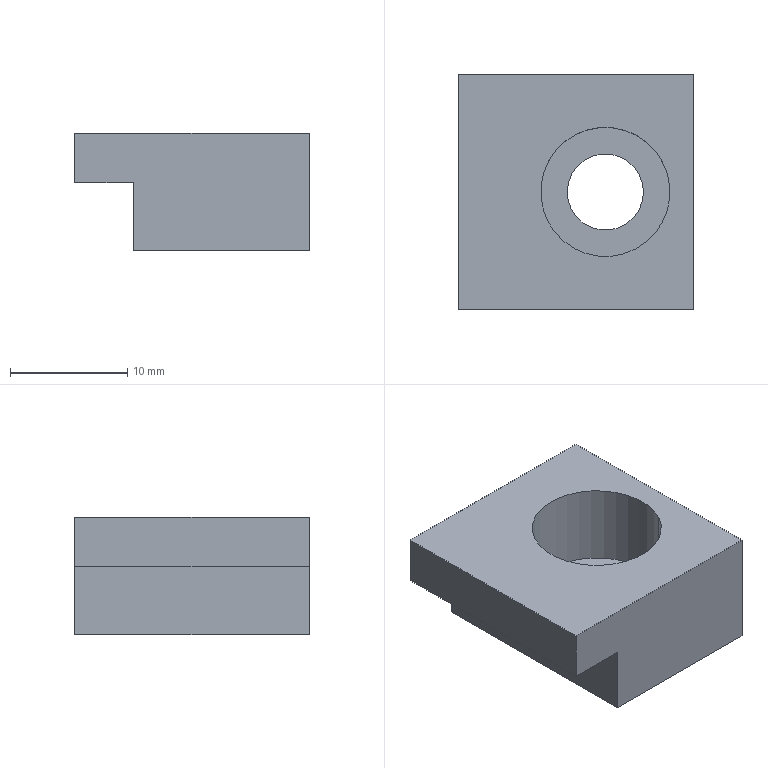Part | CATIA | 1 solid | 13 faces | box 20 x 20 x 10 mm | volume 2655 mm3 | plane 9 | cylinder 4 | commonest cylinder face diameters 6.5 x2 11 x2
STEP:
#1=CARTESIAN_POINT('',(4.827,-2.637,3.));
#2=VERTEX_POINT('',#1);
#3=CARTESIAN_POINT('',(-4.827,2.637,3.));
#4=VERTEX_POINT('',#3);
#5=CARTESIAN_POINT('',(0.,0.,3.));
#6=DIRECTION('',(0.,0.,-1.));
#7=AXIS2_PLACEMENT_3D('',#5,#6,$);
#8=CIRCLE('',#7,5.5);
#9=EDGE_CURVE('',#2,#4,#8,.T.);
#10=ORIENTED_EDGE('',*,*,#9,.F.);
#11=CARTESIAN_POINT('',(0.,0.,3.));
#12=DIRECTION('',(0.,0.,-1.));
#13=AXIS2_PLACEMENT_3D('',#11,#12,$);
#14=CIRCLE('',#13,5.5);
#15=EDGE_CURVE('',#4,#2,#14,.T.);
#16=ORIENTED_EDGE('',*,*,#15,.F.);
#17=EDGE_LOOP('',(#10,#16));
#18=FACE_OUTER_BOUND('',#17,.T.);
#19=CARTESIAN_POINT('',(-2.852,1.558,3.));
#20=VERTEX_POINT('',#19);
#21=CARTESIAN_POINT('',(2.852,-1.558,3.));
#22=VERTEX_POINT('',#21);
#23=CARTESIAN_POINT('',(0.,0.,3.));
#24=DIRECTION('',(0.,0.,-1.));
#25=AXIS2_PLACEMENT_3D('',#23,#24,$);
#26=CIRCLE('',#25,3.25);
#27=EDGE_CURVE('',#20,#22,#26,.T.);
#28=ORIENTED_EDGE('',*,*,#27,.T.);
#29=CARTESIAN_POINT('',(0.,0.,3.));
#30=DIRECTION('',(0.,0.,-1.));
#31=AXIS2_PLACEMENT_3D('',#29,#30,$);
#32=CIRCLE('',#31,3.25);
#33=EDGE_CURVE('',#22,#20,#32,.T.);
#34=ORIENTED_EDGE('',*,*,#33,.T.);
#35=EDGE_LOOP('',(#28,#34));
#36=FACE_BOUND('',#35,.T.);
#37=CARTESIAN_POINT('',(3.25,0.,3.));
#38=DIRECTION('',(0.,0.,-1.));
#39=DIRECTION('',(1.,0.,0.));
#40=AXIS2_PLACEMENT_3D('',#37,#38,#39);
#41=PLANE('',#40);
#42=ADVANCED_FACE('',(#18,#36),#41,.F.);
#43=CARTESIAN_POINT('',(-2.852,1.558,0.));
#44=VERTEX_POINT('',#43);
#45=CARTESIAN_POINT('',(2.852,-1.558,0.));
#46=VERTEX_POINT('',#45);
#47=CARTESIAN_POINT('',(0.,0.,0.));
#48=DIRECTION('',(0.,0.,-1.));
#49=AXIS2_PLACEMENT_3D('',#47,#48,$);
#50=CIRCLE('',#49,3.25);
#51=EDGE_CURVE('',#44,#46,#50,.F.);
#52=ORIENTED_EDGE('',*,*,#51,.F.);
#53=CARTESIAN_POINT('',(-2.852,1.558,-3.5));
#54=DIRECTION('',(0.,0.,-1.));
#55=VECTOR('',#54,1.);
#56=LINE('',#53,#55);
#57=EDGE_CURVE('',#44,#20,#56,.F.);
#58=ORIENTED_EDGE('',*,*,#57,.T.);
#59=ORIENTED_EDGE('',*,*,#33,.F.);
#60=CARTESIAN_POINT('',(2.852,-1.558,-3.5));
#61=DIRECTION('',(0.,0.,-1.));
#62=VECTOR('',#61,1.);
#63=LINE('',#60,#62);
#64=EDGE_CURVE('',#46,#22,#63,.F.);
#65=ORIENTED_EDGE('',*,*,#64,.F.);
#66=EDGE_LOOP('',(#52,#58,#59,#65));
#67=FACE_OUTER_BOUND('',#66,.T.);
#68=CARTESIAN_POINT('',(0.,0.,9.9));
#69=DIRECTION('',(0.,0.,-1.));
#70=DIRECTION('',(0.8776,-0.4794,0.));
#71=AXIS2_PLACEMENT_3D('',#68,#69,#70);
#72=CYLINDRICAL_SURFACE('',#71,3.25);
#73=ADVANCED_FACE('',(#67),#72,.F.);
#74=CARTESIAN_POINT('',(0.,0.,0.));
#75=DIRECTION('',(0.,0.,-1.));
#76=AXIS2_PLACEMENT_3D('',#74,#75,$);
#77=CIRCLE('',#76,3.25);
#78=EDGE_CURVE('',#46,#44,#77,.F.);
#79=ORIENTED_EDGE('',*,*,#78,.F.);
#80=ORIENTED_EDGE('',*,*,#64,.T.);
#81=ORIENTED_EDGE('',*,*,#27,.F.);
#82=ORIENTED_EDGE('',*,*,#57,.F.);
#83=EDGE_LOOP('',(#79,#80,#81,#82));
#84=FACE_OUTER_BOUND('',#83,.T.);
#85=ADVANCED_FACE('',(#84),#72,.F.);
#86=CARTESIAN_POINT('',(7.5,-10.,10.));
#87=VERTEX_POINT('',#86);
#88=CARTESIAN_POINT('',(7.5,10.,10.));
#89=VERTEX_POINT('',#88);
#90=CARTESIAN_POINT('',(7.5,0.,10.));
#91=DIRECTION('',(0.,-1.,0.));
#92=VECTOR('',#91,1.);
#93=LINE('',#90,#92);
#94=EDGE_CURVE('',#87,#89,#93,.F.);
#95=ORIENTED_EDGE('',*,*,#94,.T.);
#96=CARTESIAN_POINT('',(-12.5,10.,10.));
#97=VERTEX_POINT('',#96);
#98=CARTESIAN_POINT('',(-2.5,10.,10.));
#99=DIRECTION('',(-1.,0.,0.));
#100=VECTOR('',#99,1.);
#101=LINE('',#98,#100);
#102=EDGE_CURVE('',#89,#97,#101,.T.);
#103=ORIENTED_EDGE('',*,*,#102,.T.);
#104=CARTESIAN_POINT('',(-12.5,-10.,10.));
#105=VERTEX_POINT('',#104);
#106=CARTESIAN_POINT('',(-12.5,0.,10.));
#107=DIRECTION('',(0.,1.,0.));
#108=VECTOR('',#107,1.);
#109=LINE('',#106,#108);
#110=EDGE_CURVE('',#97,#105,#109,.F.);
#111=ORIENTED_EDGE('',*,*,#110,.T.);
#112=CARTESIAN_POINT('',(-2.5,-10.,10.));
#113=DIRECTION('',(1.,0.,0.));
#114=VECTOR('',#113,1.);
#115=LINE('',#112,#114);
#116=EDGE_CURVE('',#105,#87,#115,.T.);
#117=ORIENTED_EDGE('',*,*,#116,.T.);
#118=EDGE_LOOP('',(#95,#103,#111,#117));
#119=FACE_OUTER_BOUND('',#118,.T.);
#120=CARTESIAN_POINT('',(-4.827,2.637,10.));
#121=VERTEX_POINT('',#120);
#122=CARTESIAN_POINT('',(4.827,-2.637,10.));
#123=VERTEX_POINT('',#122);
#124=CARTESIAN_POINT('',(0.,0.,10.));
#125=DIRECTION('',(0.,0.,1.));
#126=AXIS2_PLACEMENT_3D('',#124,#125,$);
#127=CIRCLE('',#126,5.5);
#128=EDGE_CURVE('',#121,#123,#127,.T.);
#129=ORIENTED_EDGE('',*,*,#128,.F.);
#130=CARTESIAN_POINT('',(0.,0.,10.));
#131=DIRECTION('',(0.,0.,1.));
#132=AXIS2_PLACEMENT_3D('',#130,#131,$);
#133=CIRCLE('',#132,5.5);
#134=EDGE_CURVE('',#123,#121,#133,.T.);
#135=ORIENTED_EDGE('',*,*,#134,.F.);
#136=EDGE_LOOP('',(#129,#135));
#137=FACE_BOUND('',#136,.T.);
#138=CARTESIAN_POINT('',(0.,0.,10.));
#139=DIRECTION('',(0.,0.,1.));
#140=DIRECTION('',(1.,0.,0.));
#141=AXIS2_PLACEMENT_3D('',#138,#139,#140);
#142=PLANE('',#141);
#143=ADVANCED_FACE('',(#119,#137),#142,.T.);
#144=CARTESIAN_POINT('',(7.5,-10.,0.));
#145=VERTEX_POINT('',#144);
#146=CARTESIAN_POINT('',(7.5,-10.,5.));
#147=DIRECTION('',(0.,0.,1.));
#148=VECTOR('',#147,1.);
#149=LINE('',#146,#148);
#150=EDGE_CURVE('',#145,#87,#149,.T.);
#151=ORIENTED_EDGE('',*,*,#150,.F.);
#152=CARTESIAN_POINT('',(7.5,10.,0.));
#153=VERTEX_POINT('',#152);
#154=CARTESIAN_POINT('',(7.5,0.,0.));
#155=DIRECTION('',(0.,-1.,0.));
#156=VECTOR('',#155,1.);
#157=LINE('',#154,#156);
#158=EDGE_CURVE('',#145,#153,#157,.F.);
#159=ORIENTED_EDGE('',*,*,#158,.T.);
#160=CARTESIAN_POINT('',(7.5,10.,5.));
#161=DIRECTION('',(0.,0.,1.));
#162=VECTOR('',#161,1.);
#163=LINE('',#160,#162);
#164=EDGE_CURVE('',#153,#89,#163,.T.);
#165=ORIENTED_EDGE('',*,*,#164,.T.);
#166=ORIENTED_EDGE('',*,*,#94,.F.);
#167=EDGE_LOOP('',(#151,#159,#165,#166));
#168=FACE_OUTER_BOUND('',#167,.T.);
#169=CARTESIAN_POINT('',(7.5,10.,0.));
#170=DIRECTION('',(-1.,0.,0.));
#171=DIRECTION('',(0.,-1.,0.));
#172=AXIS2_PLACEMENT_3D('',#169,#170,#171);
#173=PLANE('',#172);
#174=ADVANCED_FACE('',(#168),#173,.F.);
#175=CARTESIAN_POINT('',(-12.5,10.,5.8));
#176=VERTEX_POINT('',#175);
#177=CARTESIAN_POINT('',(-12.5,10.,7.9));
#178=DIRECTION('',(0.,0.,1.));
#179=VECTOR('',#178,1.);
#180=LINE('',#177,#179);
#181=EDGE_CURVE('',#176,#97,#180,.T.);
#182=ORIENTED_EDGE('',*,*,#181,.T.);
#183=ORIENTED_EDGE('',*,*,#102,.F.);
#184=ORIENTED_EDGE('',*,*,#164,.F.);
#185=CARTESIAN_POINT('',(-7.5,10.,0.));
#186=VERTEX_POINT('',#185);
#187=CARTESIAN_POINT('',(0.,10.,0.));
#188=DIRECTION('',(-1.,0.,0.));
#189=VECTOR('',#188,1.);
#190=LINE('',#187,#189);
#191=EDGE_CURVE('',#153,#186,#190,.T.);
#192=ORIENTED_EDGE('',*,*,#191,.T.);
#193=CARTESIAN_POINT('',(-7.5,10.,5.8));
#194=VERTEX_POINT('',#193);
#195=CARTESIAN_POINT('',(-7.5,10.,2.9));
#196=DIRECTION('',(0.,0.,1.));
#197=VECTOR('',#196,1.);
#198=LINE('',#195,#197);
#199=EDGE_CURVE('',#186,#194,#198,.T.);
#200=ORIENTED_EDGE('',*,*,#199,.T.);
#201=CARTESIAN_POINT('',(-10.,10.,5.8));
#202=DIRECTION('',(1.,0.,0.));
#203=VECTOR('',#202,1.);
#204=LINE('',#201,#203);
#205=EDGE_CURVE('',#176,#194,#204,.T.);
#206=ORIENTED_EDGE('',*,*,#205,.F.);
#207=EDGE_LOOP('',(#182,#183,#184,#192,#200,#206));
#208=FACE_OUTER_BOUND('',#207,.T.);
#209=CARTESIAN_POINT('',(7.5,10.,0.));
#210=DIRECTION('',(0.,1.,0.));
#211=DIRECTION('',(-1.,0.,0.));
#212=AXIS2_PLACEMENT_3D('',#209,#210,#211);
#213=PLANE('',#212);
#214=ADVANCED_FACE('',(#208),#213,.T.);
#215=CARTESIAN_POINT('',(-12.5,-10.,5.8));
#216=VERTEX_POINT('',#215);
#217=CARTESIAN_POINT('',(-12.5,0.,5.8));
#218=DIRECTION('',(0.,1.,0.));
#219=VECTOR('',#218,1.);
#220=LINE('',#217,#219);
#221=EDGE_CURVE('',#216,#176,#220,.T.);
#222=ORIENTED_EDGE('',*,*,#221,.F.);
#223=CARTESIAN_POINT('',(-12.5,-10.,7.9));
#224=DIRECTION('',(0.,0.,1.));
#225=VECTOR('',#224,1.);
#226=LINE('',#223,#225);
#227=EDGE_CURVE('',#216,#105,#226,.T.);
#228=ORIENTED_EDGE('',*,*,#227,.T.);
#229=ORIENTED_EDGE('',*,*,#110,.F.);
#230=ORIENTED_EDGE('',*,*,#181,.F.);
#231=EDGE_LOOP('',(#222,#228,#229,#230));
#232=FACE_OUTER_BOUND('',#231,.T.);
#233=CARTESIAN_POINT('',(-12.5,-10.,0.));
#234=DIRECTION('',(1.,0.,0.));
#235=DIRECTION('',(0.,1.,0.));
#236=AXIS2_PLACEMENT_3D('',#233,#234,#235);
#237=PLANE('',#236);
#238=ADVANCED_FACE('',(#232),#237,.F.);
#239=CARTESIAN_POINT('',(-7.5,-10.,0.));
#240=VERTEX_POINT('',#239);
#241=CARTESIAN_POINT('',(0.,-10.,0.));
#242=DIRECTION('',(1.,0.,0.));
#243=VECTOR('',#242,1.);
#244=LINE('',#241,#243);
#245=EDGE_CURVE('',#240,#145,#244,.T.);
#246=ORIENTED_EDGE('',*,*,#245,.T.);
#247=ORIENTED_EDGE('',*,*,#150,.T.);
#248=ORIENTED_EDGE('',*,*,#116,.F.);
#249=ORIENTED_EDGE('',*,*,#227,.F.);
#250=CARTESIAN_POINT('',(-7.5,-10.,5.8));
#251=VERTEX_POINT('',#250);
#252=CARTESIAN_POINT('',(-10.,-10.,5.8));
#253=DIRECTION('',(1.,0.,0.));
#254=VECTOR('',#253,1.);
#255=LINE('',#252,#254);
#256=EDGE_CURVE('',#216,#251,#255,.T.);
#257=ORIENTED_EDGE('',*,*,#256,.T.);
#258=CARTESIAN_POINT('',(-7.5,-10.,2.9));
#259=DIRECTION('',(0.,0.,1.));
#260=VECTOR('',#259,1.);
#261=LINE('',#258,#260);
#262=EDGE_CURVE('',#240,#251,#261,.T.);
#263=ORIENTED_EDGE('',*,*,#262,.F.);
#264=EDGE_LOOP('',(#246,#247,#248,#249,#257,#263));
#265=FACE_OUTER_BOUND('',#264,.T.);
#266=CARTESIAN_POINT('',(-12.5,-10.,0.));
#267=DIRECTION('',(0.,-1.,0.));
#268=DIRECTION('',(1.,0.,0.));
#269=AXIS2_PLACEMENT_3D('',#266,#267,#268);
#270=PLANE('',#269);
#271=ADVANCED_FACE('',(#265),#270,.T.);
#272=ORIENTED_EDGE('',*,*,#199,.F.);
#273=CARTESIAN_POINT('',(-7.5,0.,0.));
#274=DIRECTION('',(0.,-1.,0.));
#275=VECTOR('',#274,1.);
#276=LINE('',#273,#275);
#277=EDGE_CURVE('',#186,#240,#276,.T.);
#278=ORIENTED_EDGE('',*,*,#277,.T.);
#279=ORIENTED_EDGE('',*,*,#262,.T.);
#280=CARTESIAN_POINT('',(-7.5,0.,5.8));
#281=DIRECTION('',(0.,-1.,0.));
#282=VECTOR('',#281,1.);
#283=LINE('',#280,#282);
#284=EDGE_CURVE('',#194,#251,#283,.T.);
#285=ORIENTED_EDGE('',*,*,#284,.F.);
#286=EDGE_LOOP('',(#272,#278,#279,#285));
#287=FACE_OUTER_BOUND('',#286,.T.);
#288=CARTESIAN_POINT('',(-7.5,0.,-4.2));
#289=DIRECTION('',(1.,0.,0.));
#290=DIRECTION('',(0.,0.,1.));
#291=AXIS2_PLACEMENT_3D('',#288,#289,#290);
#292=PLANE('',#291);
#293=ADVANCED_FACE('',(#287),#292,.F.);
#294=ORIENTED_EDGE('',*,*,#284,.T.);
#295=ORIENTED_EDGE('',*,*,#256,.F.);
#296=ORIENTED_EDGE('',*,*,#221,.T.);
#297=ORIENTED_EDGE('',*,*,#205,.T.);
#298=EDGE_LOOP('',(#294,#295,#296,#297));
#299=FACE_OUTER_BOUND('',#298,.T.);
#300=CARTESIAN_POINT('',(-17.5,0.,5.8));
#301=DIRECTION('',(0.,0.,-1.));
#302=DIRECTION('',(1.,0.,0.));
#303=AXIS2_PLACEMENT_3D('',#300,#301,#302);
#304=PLANE('',#303);
#305=ADVANCED_FACE('',(#299),#304,.T.);
#306=ORIENTED_EDGE('',*,*,#277,.F.);
#307=ORIENTED_EDGE('',*,*,#191,.F.);
#308=ORIENTED_EDGE('',*,*,#158,.F.);
#309=ORIENTED_EDGE('',*,*,#245,.F.);
#310=EDGE_LOOP('',(#306,#307,#308,#309));
#311=FACE_OUTER_BOUND('',#310,.T.);
#312=ORIENTED_EDGE('',*,*,#78,.T.);
#313=ORIENTED_EDGE('',*,*,#51,.T.);
#314=EDGE_LOOP('',(#312,#313));
#315=FACE_BOUND('',#314,.T.);
#316=CARTESIAN_POINT('',(0.,0.,0.));
#317=DIRECTION('',(0.,0.,1.));
#318=DIRECTION('',(1.,0.,0.));
#319=AXIS2_PLACEMENT_3D('',#316,#317,#318);
#320=PLANE('',#319);
#321=ADVANCED_FACE('',(#311,#315),#320,.F.);
#322=ORIENTED_EDGE('',*,*,#128,.T.);
#323=CARTESIAN_POINT('',(4.827,-2.637,6.655));
#324=DIRECTION('',(0.,0.,-1.));
#325=VECTOR('',#324,1.);
#326=LINE('',#323,#325);
#327=EDGE_CURVE('',#2,#123,#326,.F.);
#328=ORIENTED_EDGE('',*,*,#327,.F.);
#329=ORIENTED_EDGE('',*,*,#9,.T.);
#330=CARTESIAN_POINT('',(-4.827,2.637,6.655));
#331=DIRECTION('',(0.,0.,-1.));
#332=VECTOR('',#331,1.);
#333=LINE('',#330,#332);
#334=EDGE_CURVE('',#4,#121,#333,.F.);
#335=ORIENTED_EDGE('',*,*,#334,.T.);
#336=EDGE_LOOP('',(#322,#328,#329,#335));
#337=FACE_OUTER_BOUND('',#336,.T.);
#338=CARTESIAN_POINT('',(0.,0.,9.9));
#339=DIRECTION('',(0.,0.,-1.));
#340=DIRECTION('',(0.8776,-0.4794,0.));
#341=AXIS2_PLACEMENT_3D('',#338,#339,#340);
#342=CYLINDRICAL_SURFACE('',#341,5.5);
#343=ADVANCED_FACE('',(#337),#342,.F.);
#344=ORIENTED_EDGE('',*,*,#134,.T.);
#345=ORIENTED_EDGE('',*,*,#334,.F.);
#346=ORIENTED_EDGE('',*,*,#15,.T.);
#347=ORIENTED_EDGE('',*,*,#327,.T.);
#348=EDGE_LOOP('',(#344,#345,#346,#347));
#349=FACE_OUTER_BOUND('',#348,.T.);
#350=ADVANCED_FACE('',(#349),#342,.F.);
#351=CLOSED_SHELL('',(#42,#73,#85,#143,#174,#214,#238,#271,#293,#305,#321,#343,#350));
#352=MANIFOLD_SOLID_BREP('',#351);
#353=(LENGTH_UNIT()NAMED_UNIT(*)SI_UNIT(.MILLI.,.METRE.));
#354=UNCERTAINTY_MEASURE_WITH_UNIT(LENGTH_MEASURE(0.005),#353,'','');
#355=(NAMED_UNIT(*)PLANE_ANGLE_UNIT()SI_UNIT($,.RADIAN.));
#356=(NAMED_UNIT(*)SI_UNIT($,.STERADIAN.)SOLID_ANGLE_UNIT());
#357=(GEOMETRIC_REPRESENTATION_CONTEXT(3)GLOBAL_UNCERTAINTY_ASSIGNED_CONTEXT((#354))GLOBAL_UNIT_ASSIGNED_CONTEXT((#353,#355,#356))REPRESENTATION_CONTEXT('',''));
#358=ADVANCED_BREP_SHAPE_REPRESENTATION('',(#352),#357);